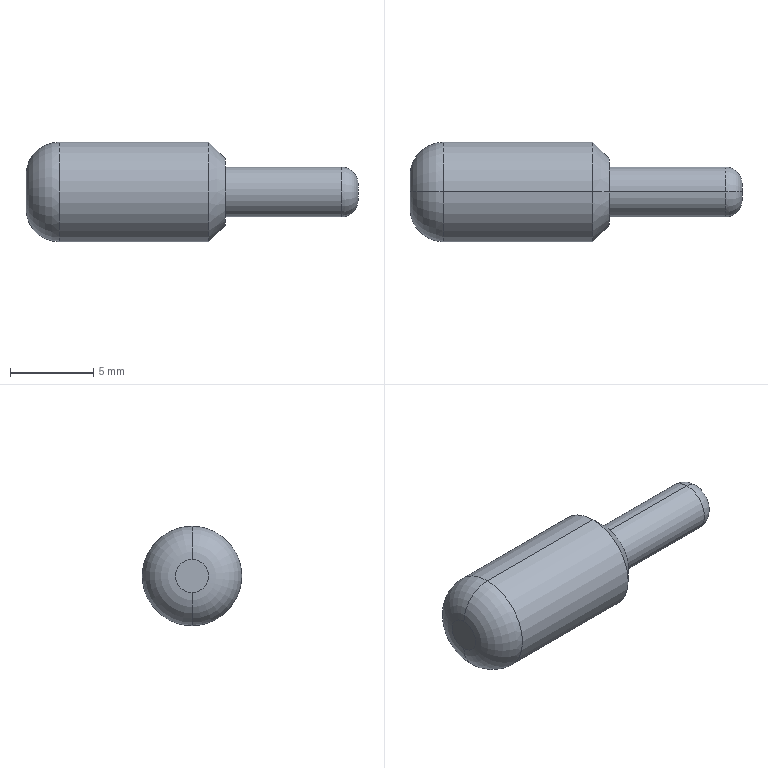Part | SolidWorks | features Fillet 2, Chamfer 1, Revolution 1 | 1 solid | 13 faces | box 20 x 6 x 6 mm | volume 371.971 mm3 | torus 4 | cylinder 4 | plane 3 | cone 2 | commonest cylinder face diameters 3 x2 6 x2
STEP:
#1=CARTESIAN_POINT('',(12.,0.,-2.));
#2=VERTEX_POINT('',#1);
#3=CARTESIAN_POINT('',(12.,0.,2.));
#4=VERTEX_POINT('',#3);
#5=CARTESIAN_POINT('',(12.,0.,0.));
#6=DIRECTION('',(1.,0.,0.));
#7=DIRECTION('',(0.,0.,1.));
#8=AXIS2_PLACEMENT_3D('',#5,#6,#7);
#9=CIRCLE('',#8,2.);
#10=EDGE_CURVE('',#2,#4,#9,.T.);
#11=ORIENTED_EDGE('',*,*,#10,.F.);
#12=CARTESIAN_POINT('',(11.,0.,-3.));
#13=VERTEX_POINT('',#12);
#14=CARTESIAN_POINT('',(11.,0.,-3.));
#15=DIRECTION('',(-0.7071,0.,-0.7071));
#16=VECTOR('',#15,1000.);
#17=LINE('',#14,#16);
#18=EDGE_CURVE('',#2,#13,#17,.T.);
#19=ORIENTED_EDGE('',*,*,#18,.T.);
#20=CARTESIAN_POINT('',(11.,0.,3.));
#21=VERTEX_POINT('',#20);
#22=CARTESIAN_POINT('',(11.,0.,0.));
#23=DIRECTION('',(-1.,0.,0.));
#24=DIRECTION('',(0.,0.,1.));
#25=AXIS2_PLACEMENT_3D('',#22,#23,#24);
#26=CIRCLE('',#25,3.);
#27=EDGE_CURVE('',#21,#13,#26,.T.);
#28=ORIENTED_EDGE('',*,*,#27,.F.);
#29=CARTESIAN_POINT('',(11.,0.,3.));
#30=DIRECTION('',(-0.7071,0.,0.7071));
#31=VECTOR('',#30,1000.);
#32=LINE('',#29,#31);
#33=EDGE_CURVE('',#4,#21,#32,.T.);
#34=ORIENTED_EDGE('',*,*,#33,.F.);
#35=EDGE_LOOP('',(#11,#19,#28,#34));
#36=FACE_OUTER_BOUND('',#35,.T.);
#37=CARTESIAN_POINT('',(11.,0.,0.));
#38=DIRECTION('',(-1.,0.,0.));
#39=DIRECTION('',(0.,0.,1.));
#40=AXIS2_PLACEMENT_3D('',#37,#38,#39);
#41=CONICAL_SURFACE('',#40,3.,0.7854);
#42=ADVANCED_FACE('',(#36),#41,.T.);
#43=CARTESIAN_POINT('',(20.,0.,-0.5));
#44=VERTEX_POINT('',#43);
#45=CARTESIAN_POINT('',(20.,0.,0.5));
#46=VERTEX_POINT('',#45);
#47=CARTESIAN_POINT('',(20.,0.,0.));
#48=DIRECTION('',(1.,0.,0.));
#49=DIRECTION('',(0.,0.,1.));
#50=AXIS2_PLACEMENT_3D('',#47,#48,#49);
#51=CIRCLE('',#50,0.5);
#52=EDGE_CURVE('',#44,#46,#51,.T.);
#53=ORIENTED_EDGE('',*,*,#52,.F.);
#54=CARTESIAN_POINT('',(19.,0.,-1.5));
#55=VERTEX_POINT('',#54);
#56=CARTESIAN_POINT('',(19.,0.,-0.5));
#57=DIRECTION('',(0.,1.,0.));
#58=DIRECTION('',(0.,0.,1.));
#59=AXIS2_PLACEMENT_3D('',#56,#57,#58);
#60=CIRCLE('',#59,1.);
#61=EDGE_CURVE('',#44,#55,#60,.T.);
#62=ORIENTED_EDGE('',*,*,#61,.T.);
#63=CARTESIAN_POINT('',(19.,0.,1.5));
#64=VERTEX_POINT('',#63);
#65=CARTESIAN_POINT('',(19.,0.,0.));
#66=DIRECTION('',(-1.,0.,0.));
#67=DIRECTION('',(0.,0.,1.));
#68=AXIS2_PLACEMENT_3D('',#65,#66,#67);
#69=CIRCLE('',#68,1.5);
#70=EDGE_CURVE('',#64,#55,#69,.T.);
#71=ORIENTED_EDGE('',*,*,#70,.F.);
#72=CARTESIAN_POINT('',(19.,0.,0.5));
#73=DIRECTION('',(0.,-1.,0.));
#74=DIRECTION('',(0.,0.,-1.));
#75=AXIS2_PLACEMENT_3D('',#72,#73,#74);
#76=CIRCLE('',#75,1.);
#77=EDGE_CURVE('',#46,#64,#76,.T.);
#78=ORIENTED_EDGE('',*,*,#77,.F.);
#79=EDGE_LOOP('',(#53,#62,#71,#78));
#80=FACE_OUTER_BOUND('',#79,.T.);
#81=CARTESIAN_POINT('',(19.,0.,0.));
#82=DIRECTION('',(-1.,0.,0.));
#83=DIRECTION('',(0.,0.,1.));
#84=AXIS2_PLACEMENT_3D('',#81,#82,#83);
#85=TOROIDAL_SURFACE('',#84,0.5,1.);
#86=ADVANCED_FACE('',(#80),#85,.T.);
#87=CARTESIAN_POINT('',(0.,0.,1.));
#88=VERTEX_POINT('',#87);
#89=CARTESIAN_POINT('',(0.,0.,-1.));
#90=VERTEX_POINT('',#89);
#91=CARTESIAN_POINT('',(0.,0.,0.));
#92=DIRECTION('',(-1.,0.,0.));
#93=DIRECTION('',(0.,0.,-1.));
#94=AXIS2_PLACEMENT_3D('',#91,#92,#93);
#95=CIRCLE('',#94,1.);
#96=EDGE_CURVE('',#88,#90,#95,.T.);
#97=ORIENTED_EDGE('',*,*,#96,.F.);
#98=CARTESIAN_POINT('',(2.,0.,3.));
#99=VERTEX_POINT('',#98);
#100=CARTESIAN_POINT('',(2.,0.,1.));
#101=DIRECTION('',(0.,1.,0.));
#102=DIRECTION('',(0.,0.,1.));
#103=AXIS2_PLACEMENT_3D('',#100,#101,#102);
#104=CIRCLE('',#103,2.);
#105=EDGE_CURVE('',#88,#99,#104,.T.);
#106=ORIENTED_EDGE('',*,*,#105,.T.);
#107=CARTESIAN_POINT('',(2.,0.,-3.));
#108=VERTEX_POINT('',#107);
#109=CARTESIAN_POINT('',(2.,0.,0.));
#110=DIRECTION('',(1.,0.,0.));
#111=DIRECTION('',(0.,0.,-1.));
#112=AXIS2_PLACEMENT_3D('',#109,#110,#111);
#113=CIRCLE('',#112,3.);
#114=EDGE_CURVE('',#108,#99,#113,.T.);
#115=ORIENTED_EDGE('',*,*,#114,.F.);
#116=CARTESIAN_POINT('',(2.,0.,-1.));
#117=DIRECTION('',(0.,-1.,0.));
#118=DIRECTION('',(0.,0.,-1.));
#119=AXIS2_PLACEMENT_3D('',#116,#117,#118);
#120=CIRCLE('',#119,2.);
#121=EDGE_CURVE('',#90,#108,#120,.T.);
#122=ORIENTED_EDGE('',*,*,#121,.F.);
#123=EDGE_LOOP('',(#97,#106,#115,#122));
#124=FACE_OUTER_BOUND('',#123,.T.);
#125=CARTESIAN_POINT('',(2.,0.,0.));
#126=DIRECTION('',(1.,0.,0.));
#127=DIRECTION('',(0.,0.,-1.));
#128=AXIS2_PLACEMENT_3D('',#125,#126,#127);
#129=TOROIDAL_SURFACE('',#128,1.,2.);
#130=ADVANCED_FACE('',(#124),#129,.T.);
#131=ORIENTED_EDGE('',*,*,#70,.T.);
#132=CARTESIAN_POINT('',(12.,0.,-1.5));
#133=VERTEX_POINT('',#132);
#134=CARTESIAN_POINT('',(0.,0.,-1.5));
#135=DIRECTION('',(-1.,0.,0.));
#136=VECTOR('',#135,1000.);
#137=LINE('',#134,#136);
#138=EDGE_CURVE('',#55,#133,#137,.T.);
#139=ORIENTED_EDGE('',*,*,#138,.T.);
#140=CARTESIAN_POINT('',(12.,0.,1.5));
#141=VERTEX_POINT('',#140);
#142=CARTESIAN_POINT('',(12.,0.,0.));
#143=DIRECTION('',(-1.,0.,0.));
#144=DIRECTION('',(0.,0.,1.));
#145=AXIS2_PLACEMENT_3D('',#142,#143,#144);
#146=CIRCLE('',#145,1.5);
#147=EDGE_CURVE('',#141,#133,#146,.T.);
#148=ORIENTED_EDGE('',*,*,#147,.F.);
#149=CARTESIAN_POINT('',(0.,0.,1.5));
#150=DIRECTION('',(-1.,0.,0.));
#151=VECTOR('',#150,1000.);
#152=LINE('',#149,#151);
#153=EDGE_CURVE('',#64,#141,#152,.T.);
#154=ORIENTED_EDGE('',*,*,#153,.F.);
#155=EDGE_LOOP('',(#131,#139,#148,#154));
#156=FACE_OUTER_BOUND('',#155,.T.);
#157=CARTESIAN_POINT('',(0.,0.,0.));
#158=DIRECTION('',(-1.,0.,0.));
#159=DIRECTION('',(0.,0.,1.));
#160=AXIS2_PLACEMENT_3D('',#157,#158,#159);
#161=CYLINDRICAL_SURFACE('',#160,1.5);
#162=ADVANCED_FACE('',(#156),#161,.T.);
#163=ORIENTED_EDGE('',*,*,#27,.T.);
#164=CARTESIAN_POINT('',(0.,0.,-3.));
#165=DIRECTION('',(-1.,0.,0.));
#166=VECTOR('',#165,1000.);
#167=LINE('',#164,#166);
#168=EDGE_CURVE('',#13,#108,#167,.T.);
#169=ORIENTED_EDGE('',*,*,#168,.T.);
#170=ORIENTED_EDGE('',*,*,#114,.T.);
#171=CARTESIAN_POINT('',(0.,0.,3.));
#172=DIRECTION('',(-1.,0.,0.));
#173=VECTOR('',#172,1000.);
#174=LINE('',#171,#173);
#175=EDGE_CURVE('',#21,#99,#174,.T.);
#176=ORIENTED_EDGE('',*,*,#175,.F.);
#177=EDGE_LOOP('',(#163,#169,#170,#176));
#178=FACE_OUTER_BOUND('',#177,.T.);
#179=CARTESIAN_POINT('',(0.,0.,0.));
#180=DIRECTION('',(-1.,0.,0.));
#181=DIRECTION('',(0.,0.,1.));
#182=AXIS2_PLACEMENT_3D('',#179,#180,#181);
#183=CYLINDRICAL_SURFACE('',#182,3.);
#184=ADVANCED_FACE('',(#178),#183,.T.);
#185=CARTESIAN_POINT('',(0.,0.,0.));
#186=DIRECTION('',(-1.,0.,0.));
#187=DIRECTION('',(0.,0.,-1.));
#188=AXIS2_PLACEMENT_3D('',#185,#186,#187);
#189=CIRCLE('',#188,1.);
#190=EDGE_CURVE('',#90,#88,#189,.T.);
#191=ORIENTED_EDGE('',*,*,#190,.T.);
#192=ORIENTED_EDGE('',*,*,#96,.T.);
#193=EDGE_LOOP('',(#191,#192));
#194=FACE_OUTER_BOUND('',#193,.T.);
#195=CARTESIAN_POINT('',(0.,0.,0.));
#196=DIRECTION('',(1.,0.,0.));
#197=DIRECTION('',(0.,0.,-1.));
#198=AXIS2_PLACEMENT_3D('',#195,#196,#197);
#199=PLANE('',#198);
#200=ADVANCED_FACE('',(#194),#199,.F.);
#201=ORIENTED_EDGE('',*,*,#168,.F.);
#202=CARTESIAN_POINT('',(11.,0.,0.));
#203=DIRECTION('',(-1.,0.,0.));
#204=DIRECTION('',(0.,0.,1.));
#205=AXIS2_PLACEMENT_3D('',#202,#203,#204);
#206=CIRCLE('',#205,3.);
#207=EDGE_CURVE('',#13,#21,#206,.T.);
#208=ORIENTED_EDGE('',*,*,#207,.T.);
#209=ORIENTED_EDGE('',*,*,#175,.T.);
#210=CARTESIAN_POINT('',(2.,0.,0.));
#211=DIRECTION('',(1.,0.,0.));
#212=DIRECTION('',(0.,0.,-1.));
#213=AXIS2_PLACEMENT_3D('',#210,#211,#212);
#214=CIRCLE('',#213,3.);
#215=EDGE_CURVE('',#99,#108,#214,.T.);
#216=ORIENTED_EDGE('',*,*,#215,.T.);
#217=EDGE_LOOP('',(#201,#208,#209,#216));
#218=FACE_OUTER_BOUND('',#217,.T.);
#219=CARTESIAN_POINT('',(0.,0.,0.));
#220=DIRECTION('',(-1.,0.,0.));
#221=DIRECTION('',(0.,0.,1.));
#222=AXIS2_PLACEMENT_3D('',#219,#220,#221);
#223=CYLINDRICAL_SURFACE('',#222,3.);
#224=ADVANCED_FACE('',(#218),#223,.T.);
#225=CARTESIAN_POINT('',(12.,0.,0.));
#226=DIRECTION('',(1.,0.,0.));
#227=DIRECTION('',(0.,0.,1.));
#228=AXIS2_PLACEMENT_3D('',#225,#226,#227);
#229=CIRCLE('',#228,2.);
#230=EDGE_CURVE('',#4,#2,#229,.T.);
#231=ORIENTED_EDGE('',*,*,#230,.T.);
#232=ORIENTED_EDGE('',*,*,#10,.T.);
#233=EDGE_LOOP('',(#231,#232));
#234=FACE_OUTER_BOUND('',#233,.T.);
#235=ORIENTED_EDGE('',*,*,#147,.T.);
#236=CARTESIAN_POINT('',(12.,0.,0.));
#237=DIRECTION('',(-1.,0.,0.));
#238=DIRECTION('',(0.,0.,1.));
#239=AXIS2_PLACEMENT_3D('',#236,#237,#238);
#240=CIRCLE('',#239,1.5);
#241=EDGE_CURVE('',#133,#141,#240,.T.);
#242=ORIENTED_EDGE('',*,*,#241,.T.);
#243=EDGE_LOOP('',(#235,#242));
#244=FACE_BOUND('',#243,.T.);
#245=CARTESIAN_POINT('',(12.,3.,0.));
#246=DIRECTION('',(-1.,0.,0.));
#247=DIRECTION('',(0.,0.,1.));
#248=AXIS2_PLACEMENT_3D('',#245,#246,#247);
#249=PLANE('',#248);
#250=ADVANCED_FACE('',(#234,#244),#249,.F.);
#251=ORIENTED_EDGE('',*,*,#138,.F.);
#252=CARTESIAN_POINT('',(19.,0.,0.));
#253=DIRECTION('',(-1.,0.,0.));
#254=DIRECTION('',(0.,0.,1.));
#255=AXIS2_PLACEMENT_3D('',#252,#253,#254);
#256=CIRCLE('',#255,1.5);
#257=EDGE_CURVE('',#55,#64,#256,.T.);
#258=ORIENTED_EDGE('',*,*,#257,.T.);
#259=ORIENTED_EDGE('',*,*,#153,.T.);
#260=ORIENTED_EDGE('',*,*,#241,.F.);
#261=EDGE_LOOP('',(#251,#258,#259,#260));
#262=FACE_OUTER_BOUND('',#261,.T.);
#263=CARTESIAN_POINT('',(0.,0.,0.));
#264=DIRECTION('',(-1.,0.,0.));
#265=DIRECTION('',(0.,0.,1.));
#266=AXIS2_PLACEMENT_3D('',#263,#264,#265);
#267=CYLINDRICAL_SURFACE('',#266,1.5);
#268=ADVANCED_FACE('',(#262),#267,.T.);
#269=CARTESIAN_POINT('',(20.,0.,0.));
#270=DIRECTION('',(1.,0.,0.));
#271=DIRECTION('',(0.,0.,1.));
#272=AXIS2_PLACEMENT_3D('',#269,#270,#271);
#273=CIRCLE('',#272,0.5);
#274=EDGE_CURVE('',#46,#44,#273,.T.);
#275=ORIENTED_EDGE('',*,*,#274,.T.);
#276=ORIENTED_EDGE('',*,*,#52,.T.);
#277=EDGE_LOOP('',(#275,#276));
#278=FACE_OUTER_BOUND('',#277,.T.);
#279=CARTESIAN_POINT('',(20.,1.5,0.));
#280=DIRECTION('',(-1.,0.,0.));
#281=DIRECTION('',(0.,0.,1.));
#282=AXIS2_PLACEMENT_3D('',#279,#280,#281);
#283=PLANE('',#282);
#284=ADVANCED_FACE('',(#278),#283,.F.);
#285=ORIENTED_EDGE('',*,*,#105,.F.);
#286=ORIENTED_EDGE('',*,*,#190,.F.);
#287=ORIENTED_EDGE('',*,*,#121,.T.);
#288=ORIENTED_EDGE('',*,*,#215,.F.);
#289=EDGE_LOOP('',(#285,#286,#287,#288));
#290=FACE_OUTER_BOUND('',#289,.T.);
#291=CARTESIAN_POINT('',(2.,0.,0.));
#292=DIRECTION('',(1.,0.,0.));
#293=DIRECTION('',(0.,0.,-1.));
#294=AXIS2_PLACEMENT_3D('',#291,#292,#293);
#295=TOROIDAL_SURFACE('',#294,1.,2.);
#296=ADVANCED_FACE('',(#290),#295,.T.);
#297=ORIENTED_EDGE('',*,*,#61,.F.);
#298=ORIENTED_EDGE('',*,*,#274,.F.);
#299=ORIENTED_EDGE('',*,*,#77,.T.);
#300=ORIENTED_EDGE('',*,*,#257,.F.);
#301=EDGE_LOOP('',(#297,#298,#299,#300));
#302=FACE_OUTER_BOUND('',#301,.T.);
#303=CARTESIAN_POINT('',(19.,0.,0.));
#304=DIRECTION('',(-1.,0.,0.));
#305=DIRECTION('',(0.,0.,1.));
#306=AXIS2_PLACEMENT_3D('',#303,#304,#305);
#307=TOROIDAL_SURFACE('',#306,0.5,1.);
#308=ADVANCED_FACE('',(#302),#307,.T.);
#309=ORIENTED_EDGE('',*,*,#18,.F.);
#310=ORIENTED_EDGE('',*,*,#230,.F.);
#311=ORIENTED_EDGE('',*,*,#33,.T.);
#312=ORIENTED_EDGE('',*,*,#207,.F.);
#313=EDGE_LOOP('',(#309,#310,#311,#312));
#314=FACE_OUTER_BOUND('',#313,.T.);
#315=CARTESIAN_POINT('',(11.,0.,0.));
#316=DIRECTION('',(-1.,0.,0.));
#317=DIRECTION('',(0.,0.,1.));
#318=AXIS2_PLACEMENT_3D('',#315,#316,#317);
#319=CONICAL_SURFACE('',#318,3.,0.7854);
#320=ADVANCED_FACE('',(#314),#319,.T.);
#321=CLOSED_SHELL('',(#42,#86,#130,#162,#184,#200,#224,#250,#268,#284,#296,#308,#320));
#322=MANIFOLD_SOLID_BREP('',#321);
#323=CARTESIAN_POINT('',(0.,0.,0.));
#324=DIRECTION('',(0.,0.,1.));
#325=DIRECTION('',(1.,0.,0.));
#326=AXIS2_PLACEMENT_3D('',#323,#324,#325);
#327=(LENGTH_UNIT()NAMED_UNIT(*)SI_UNIT(.MILLI.,.METRE.));
#328=UNCERTAINTY_MEASURE_WITH_UNIT(LENGTH_MEASURE(0.00001),#327,'','');
#329=(NAMED_UNIT(*)PLANE_ANGLE_UNIT()SI_UNIT($,.RADIAN.));
#330=(NAMED_UNIT(*)SI_UNIT($,.STERADIAN.)SOLID_ANGLE_UNIT());
#331=(GEOMETRIC_REPRESENTATION_CONTEXT(3)GLOBAL_UNCERTAINTY_ASSIGNED_CONTEXT((#328))GLOBAL_UNIT_ASSIGNED_CONTEXT((#327,#329,#330))REPRESENTATION_CONTEXT('',''));
#332=ADVANCED_BREP_SHAPE_REPRESENTATION('',(#322,#326),#331);